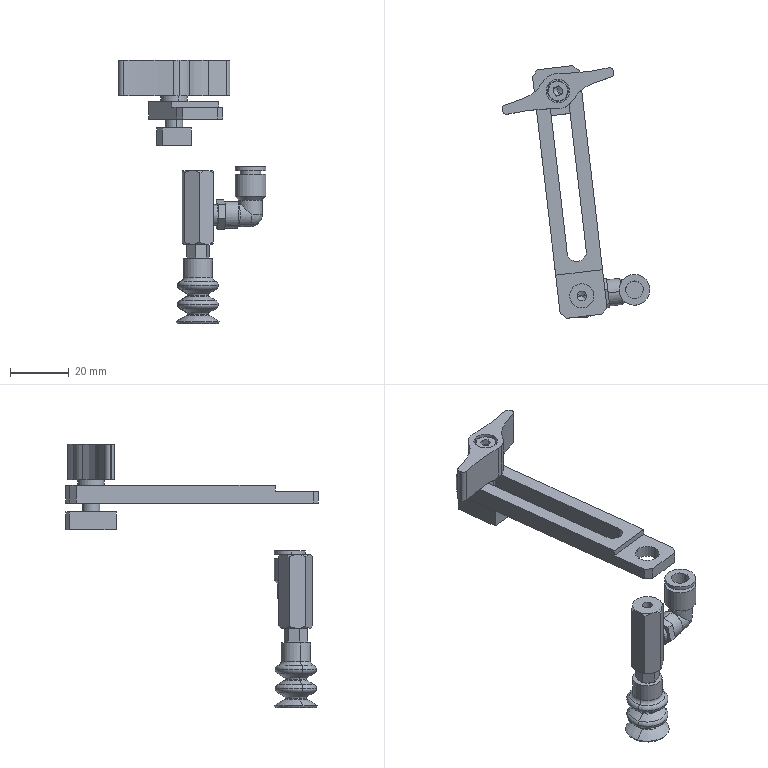Part | SolidWorks | 8 solids | 257 faces | box 50.199 x 85.818 x 89.5 mm | volume 14095 mm3 | plane 85 | cylinder 66 | cone 63 | torus 40 | sphere 3 | commonest cylinder face diameters 5 x8 2.5 x6 7 x6 8 x6 3 x4 4.2 x4